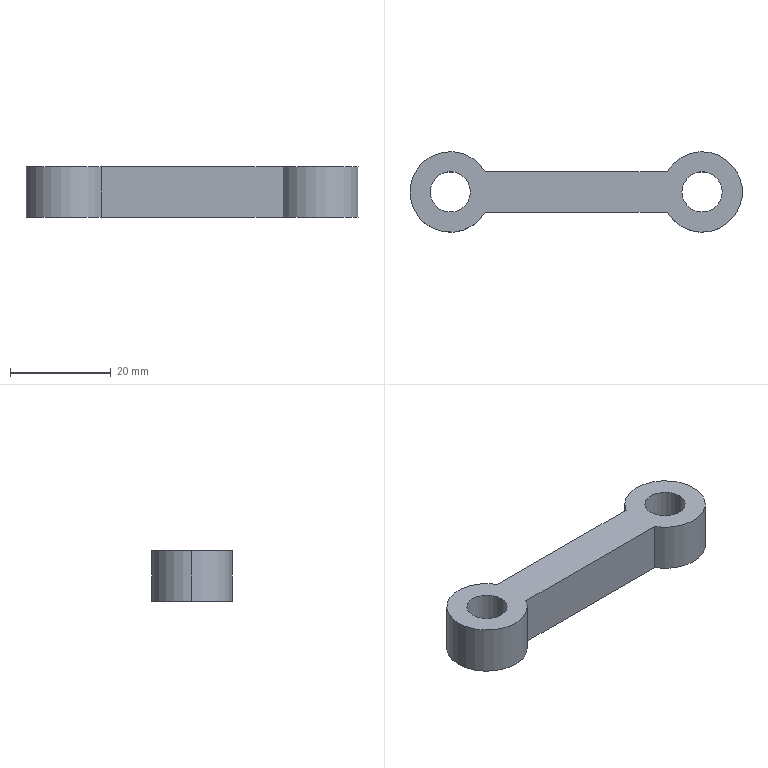Part | SolidWorks | features Extrusion 1 | 1 solid | 11 faces | box 66 x 16 x 10 mm | volume 5791 mm3 | cylinder 7 | plane 4 | commonest cylinder face diameters 8 x4 16 x3
STEP:
#1=CARTESIAN_POINT('',(46.,0.,10.));
#2=VERTEX_POINT('',#1);
#3=CARTESIAN_POINT('',(54.,0.,10.));
#4=VERTEX_POINT('',#3);
#5=CARTESIAN_POINT('',(50.,0.,10.));
#6=DIRECTION('',(0.,0.,1.));
#7=DIRECTION('',(1.,0.,0.));
#8=AXIS2_PLACEMENT_3D('',#5,#6,#7);
#9=CIRCLE('',#8,4.);
#10=EDGE_CURVE('',#2,#4,#9,.T.);
#11=ORIENTED_EDGE('',*,*,#10,.T.);
#12=CARTESIAN_POINT('',(54.,0.,0.));
#13=VERTEX_POINT('',#12);
#14=CARTESIAN_POINT('',(54.,0.,10.));
#15=DIRECTION('',(0.,0.,-1.));
#16=VECTOR('',#15,1000.);
#17=LINE('',#14,#16);
#18=EDGE_CURVE('',#4,#13,#17,.T.);
#19=ORIENTED_EDGE('',*,*,#18,.T.);
#20=CARTESIAN_POINT('',(46.,0.,0.));
#21=VERTEX_POINT('',#20);
#22=CARTESIAN_POINT('',(50.,0.,0.));
#23=DIRECTION('',(0.,0.,1.));
#24=DIRECTION('',(1.,0.,0.));
#25=AXIS2_PLACEMENT_3D('',#22,#23,#24);
#26=CIRCLE('',#25,4.);
#27=EDGE_CURVE('',#21,#13,#26,.T.);
#28=ORIENTED_EDGE('',*,*,#27,.F.);
#29=CARTESIAN_POINT('',(46.,0.,10.));
#30=DIRECTION('',(0.,0.,-1.));
#31=VECTOR('',#30,1000.);
#32=LINE('',#29,#31);
#33=EDGE_CURVE('',#2,#21,#32,.T.);
#34=ORIENTED_EDGE('',*,*,#33,.F.);
#35=EDGE_LOOP('',(#11,#19,#28,#34));
#36=FACE_OUTER_BOUND('',#35,.T.);
#37=CARTESIAN_POINT('',(50.,0.,10.));
#38=DIRECTION('',(0.,0.,-1.));
#39=DIRECTION('',(-1.,0.,0.));
#40=AXIS2_PLACEMENT_3D('',#37,#38,#39);
#41=CYLINDRICAL_SURFACE('',#40,4.);
#42=ADVANCED_FACE('',(#36),#41,.F.);
#43=CARTESIAN_POINT('',(-4.,0.,10.));
#44=VERTEX_POINT('',#43);
#45=CARTESIAN_POINT('',(4.,0.,10.));
#46=VERTEX_POINT('',#45);
#47=CARTESIAN_POINT('',(0.,0.,10.));
#48=DIRECTION('',(0.,0.,1.));
#49=DIRECTION('',(1.,0.,0.));
#50=AXIS2_PLACEMENT_3D('',#47,#48,#49);
#51=CIRCLE('',#50,4.);
#52=EDGE_CURVE('',#44,#46,#51,.T.);
#53=ORIENTED_EDGE('',*,*,#52,.T.);
#54=CARTESIAN_POINT('',(4.,0.,0.));
#55=VERTEX_POINT('',#54);
#56=CARTESIAN_POINT('',(4.,0.,10.));
#57=DIRECTION('',(0.,0.,-1.));
#58=VECTOR('',#57,1000.);
#59=LINE('',#56,#58);
#60=EDGE_CURVE('',#46,#55,#59,.T.);
#61=ORIENTED_EDGE('',*,*,#60,.T.);
#62=CARTESIAN_POINT('',(-4.,0.,0.));
#63=VERTEX_POINT('',#62);
#64=CARTESIAN_POINT('',(0.,0.,0.));
#65=DIRECTION('',(0.,0.,1.));
#66=DIRECTION('',(1.,0.,0.));
#67=AXIS2_PLACEMENT_3D('',#64,#65,#66);
#68=CIRCLE('',#67,4.);
#69=EDGE_CURVE('',#63,#55,#68,.T.);
#70=ORIENTED_EDGE('',*,*,#69,.F.);
#71=CARTESIAN_POINT('',(-4.,0.,10.));
#72=DIRECTION('',(0.,0.,-1.));
#73=VECTOR('',#72,1000.);
#74=LINE('',#71,#73);
#75=EDGE_CURVE('',#44,#63,#74,.T.);
#76=ORIENTED_EDGE('',*,*,#75,.F.);
#77=EDGE_LOOP('',(#53,#61,#70,#76));
#78=FACE_OUTER_BOUND('',#77,.T.);
#79=CARTESIAN_POINT('',(0.,0.,10.));
#80=DIRECTION('',(0.,0.,-1.));
#81=DIRECTION('',(-1.,0.,0.));
#82=AXIS2_PLACEMENT_3D('',#79,#80,#81);
#83=CYLINDRICAL_SURFACE('',#82,4.);
#84=ADVANCED_FACE('',(#78),#83,.F.);
#85=CARTESIAN_POINT('',(-8.,0.,10.));
#86=VERTEX_POINT('',#85);
#87=CARTESIAN_POINT('',(6.928,-4.,10.));
#88=VERTEX_POINT('',#87);
#89=CARTESIAN_POINT('',(0.,0.,10.));
#90=DIRECTION('',(0.,0.,1.));
#91=DIRECTION('',(1.,0.,0.));
#92=AXIS2_PLACEMENT_3D('',#89,#90,#91);
#93=CIRCLE('',#92,8.);
#94=EDGE_CURVE('',#86,#88,#93,.T.);
#95=ORIENTED_EDGE('',*,*,#94,.F.);
#96=CARTESIAN_POINT('',(-8.,0.,0.));
#97=VERTEX_POINT('',#96);
#98=CARTESIAN_POINT('',(-8.,0.,10.));
#99=DIRECTION('',(0.,0.,-1.));
#100=VECTOR('',#99,1000.);
#101=LINE('',#98,#100);
#102=EDGE_CURVE('',#86,#97,#101,.T.);
#103=ORIENTED_EDGE('',*,*,#102,.T.);
#104=CARTESIAN_POINT('',(6.928,-4.,0.));
#105=VERTEX_POINT('',#104);
#106=CARTESIAN_POINT('',(0.,0.,0.));
#107=DIRECTION('',(0.,0.,1.));
#108=DIRECTION('',(1.,0.,0.));
#109=AXIS2_PLACEMENT_3D('',#106,#107,#108);
#110=CIRCLE('',#109,8.);
#111=EDGE_CURVE('',#97,#105,#110,.T.);
#112=ORIENTED_EDGE('',*,*,#111,.T.);
#113=CARTESIAN_POINT('',(6.928,-4.,10.));
#114=DIRECTION('',(0.,0.,-1.));
#115=VECTOR('',#114,1000.);
#116=LINE('',#113,#115);
#117=EDGE_CURVE('',#88,#105,#116,.T.);
#118=ORIENTED_EDGE('',*,*,#117,.F.);
#119=EDGE_LOOP('',(#95,#103,#112,#118));
#120=FACE_OUTER_BOUND('',#119,.T.);
#121=CARTESIAN_POINT('',(0.,0.,10.));
#122=DIRECTION('',(0.,0.,-1.));
#123=DIRECTION('',(-1.,0.,0.));
#124=AXIS2_PLACEMENT_3D('',#121,#122,#123);
#125=CYLINDRICAL_SURFACE('',#124,8.);
#126=ADVANCED_FACE('',(#120),#125,.T.);
#127=ORIENTED_EDGE('',*,*,#52,.F.);
#128=CARTESIAN_POINT('',(0.,0.,10.));
#129=DIRECTION('',(0.,0.,1.));
#130=DIRECTION('',(1.,0.,0.));
#131=AXIS2_PLACEMENT_3D('',#128,#129,#130);
#132=CIRCLE('',#131,4.);
#133=EDGE_CURVE('',#46,#44,#132,.T.);
#134=ORIENTED_EDGE('',*,*,#133,.F.);
#135=EDGE_LOOP('',(#127,#134));
#136=FACE_BOUND('',#135,.T.);
#137=CARTESIAN_POINT('',(6.928,4.,10.));
#138=VERTEX_POINT('',#137);
#139=CARTESIAN_POINT('',(0.,0.,10.));
#140=DIRECTION('',(0.,0.,1.));
#141=DIRECTION('',(1.,0.,0.));
#142=AXIS2_PLACEMENT_3D('',#139,#140,#141);
#143=CIRCLE('',#142,8.);
#144=EDGE_CURVE('',#138,#86,#143,.T.);
#145=ORIENTED_EDGE('',*,*,#144,.T.);
#146=ORIENTED_EDGE('',*,*,#94,.T.);
#147=CARTESIAN_POINT('',(43.072,-4.,10.));
#148=VERTEX_POINT('',#147);
#149=CARTESIAN_POINT('',(6.928,-4.,10.));
#150=DIRECTION('',(1.,0.,0.));
#151=VECTOR('',#150,1000.);
#152=LINE('',#149,#151);
#153=EDGE_CURVE('',#88,#148,#152,.T.);
#154=ORIENTED_EDGE('',*,*,#153,.T.);
#155=CARTESIAN_POINT('',(43.072,4.,10.));
#156=VERTEX_POINT('',#155);
#157=CARTESIAN_POINT('',(50.,0.,10.));
#158=DIRECTION('',(0.,0.,1.));
#159=DIRECTION('',(1.,0.,0.));
#160=AXIS2_PLACEMENT_3D('',#157,#158,#159);
#161=CIRCLE('',#160,8.);
#162=EDGE_CURVE('',#148,#156,#161,.T.);
#163=ORIENTED_EDGE('',*,*,#162,.T.);
#164=CARTESIAN_POINT('',(6.928,4.,10.));
#165=DIRECTION('',(-1.,0.,0.));
#166=VECTOR('',#165,1000.);
#167=LINE('',#164,#166);
#168=EDGE_CURVE('',#156,#138,#167,.T.);
#169=ORIENTED_EDGE('',*,*,#168,.T.);
#170=EDGE_LOOP('',(#145,#146,#154,#163,#169));
#171=FACE_OUTER_BOUND('',#170,.T.);
#172=ORIENTED_EDGE('',*,*,#10,.F.);
#173=CARTESIAN_POINT('',(50.,0.,10.));
#174=DIRECTION('',(0.,0.,1.));
#175=DIRECTION('',(1.,0.,0.));
#176=AXIS2_PLACEMENT_3D('',#173,#174,#175);
#177=CIRCLE('',#176,4.);
#178=EDGE_CURVE('',#4,#2,#177,.T.);
#179=ORIENTED_EDGE('',*,*,#178,.F.);
#180=EDGE_LOOP('',(#172,#179));
#181=FACE_BOUND('',#180,.T.);
#182=CARTESIAN_POINT('',(0.,0.,10.));
#183=DIRECTION('',(0.,0.,1.));
#184=DIRECTION('',(1.,0.,0.));
#185=AXIS2_PLACEMENT_3D('',#182,#183,#184);
#186=PLANE('',#185);
#187=ADVANCED_FACE('',(#136,#171,#181),#186,.T.);
#188=CARTESIAN_POINT('',(6.928,4.,0.));
#189=VERTEX_POINT('',#188);
#190=CARTESIAN_POINT('',(0.,0.,0.));
#191=DIRECTION('',(0.,0.,1.));
#192=DIRECTION('',(1.,0.,0.));
#193=AXIS2_PLACEMENT_3D('',#190,#191,#192);
#194=CIRCLE('',#193,8.);
#195=EDGE_CURVE('',#189,#97,#194,.T.);
#196=ORIENTED_EDGE('',*,*,#195,.F.);
#197=CARTESIAN_POINT('',(43.072,4.,0.));
#198=VERTEX_POINT('',#197);
#199=CARTESIAN_POINT('',(6.928,4.,0.));
#200=DIRECTION('',(-1.,0.,0.));
#201=VECTOR('',#200,1000.);
#202=LINE('',#199,#201);
#203=EDGE_CURVE('',#198,#189,#202,.T.);
#204=ORIENTED_EDGE('',*,*,#203,.F.);
#205=CARTESIAN_POINT('',(43.072,-4.,0.));
#206=VERTEX_POINT('',#205);
#207=CARTESIAN_POINT('',(50.,0.,0.));
#208=DIRECTION('',(0.,0.,1.));
#209=DIRECTION('',(1.,0.,0.));
#210=AXIS2_PLACEMENT_3D('',#207,#208,#209);
#211=CIRCLE('',#210,8.);
#212=EDGE_CURVE('',#206,#198,#211,.T.);
#213=ORIENTED_EDGE('',*,*,#212,.F.);
#214=CARTESIAN_POINT('',(6.928,-4.,0.));
#215=DIRECTION('',(1.,0.,0.));
#216=VECTOR('',#215,1000.);
#217=LINE('',#214,#216);
#218=EDGE_CURVE('',#105,#206,#217,.T.);
#219=ORIENTED_EDGE('',*,*,#218,.F.);
#220=ORIENTED_EDGE('',*,*,#111,.F.);
#221=EDGE_LOOP('',(#196,#204,#213,#219,#220));
#222=FACE_OUTER_BOUND('',#221,.T.);
#223=ORIENTED_EDGE('',*,*,#69,.T.);
#224=CARTESIAN_POINT('',(0.,0.,0.));
#225=DIRECTION('',(0.,0.,1.));
#226=DIRECTION('',(1.,0.,0.));
#227=AXIS2_PLACEMENT_3D('',#224,#225,#226);
#228=CIRCLE('',#227,4.);
#229=EDGE_CURVE('',#55,#63,#228,.T.);
#230=ORIENTED_EDGE('',*,*,#229,.T.);
#231=EDGE_LOOP('',(#223,#230));
#232=FACE_BOUND('',#231,.T.);
#233=ORIENTED_EDGE('',*,*,#27,.T.);
#234=CARTESIAN_POINT('',(50.,0.,0.));
#235=DIRECTION('',(0.,0.,1.));
#236=DIRECTION('',(1.,0.,0.));
#237=AXIS2_PLACEMENT_3D('',#234,#235,#236);
#238=CIRCLE('',#237,4.);
#239=EDGE_CURVE('',#13,#21,#238,.T.);
#240=ORIENTED_EDGE('',*,*,#239,.T.);
#241=EDGE_LOOP('',(#233,#240));
#242=FACE_BOUND('',#241,.T.);
#243=CARTESIAN_POINT('',(0.,0.,0.));
#244=DIRECTION('',(0.,0.,1.));
#245=DIRECTION('',(1.,0.,0.));
#246=AXIS2_PLACEMENT_3D('',#243,#244,#245);
#247=PLANE('',#246);
#248=ADVANCED_FACE('',(#222,#232,#242),#247,.F.);
#249=ORIENTED_EDGE('',*,*,#102,.F.);
#250=ORIENTED_EDGE('',*,*,#144,.F.);
#251=CARTESIAN_POINT('',(6.928,4.,10.));
#252=DIRECTION('',(0.,0.,-1.));
#253=VECTOR('',#252,1000.);
#254=LINE('',#251,#253);
#255=EDGE_CURVE('',#138,#189,#254,.T.);
#256=ORIENTED_EDGE('',*,*,#255,.T.);
#257=ORIENTED_EDGE('',*,*,#195,.T.);
#258=EDGE_LOOP('',(#249,#250,#256,#257));
#259=FACE_OUTER_BOUND('',#258,.T.);
#260=CARTESIAN_POINT('',(0.,0.,10.));
#261=DIRECTION('',(0.,0.,-1.));
#262=DIRECTION('',(-1.,0.,0.));
#263=AXIS2_PLACEMENT_3D('',#260,#261,#262);
#264=CYLINDRICAL_SURFACE('',#263,8.);
#265=ADVANCED_FACE('',(#259),#264,.T.);
#266=ORIENTED_EDGE('',*,*,#218,.T.);
#267=CARTESIAN_POINT('',(43.072,-4.,10.));
#268=DIRECTION('',(0.,0.,-1.));
#269=VECTOR('',#268,1000.);
#270=LINE('',#267,#269);
#271=EDGE_CURVE('',#148,#206,#270,.T.);
#272=ORIENTED_EDGE('',*,*,#271,.F.);
#273=ORIENTED_EDGE('',*,*,#153,.F.);
#274=ORIENTED_EDGE('',*,*,#117,.T.);
#275=EDGE_LOOP('',(#266,#272,#273,#274));
#276=FACE_OUTER_BOUND('',#275,.T.);
#277=CARTESIAN_POINT('',(6.928,-4.,10.));
#278=DIRECTION('',(0.,1.,0.));
#279=DIRECTION('',(0.,0.,1.));
#280=AXIS2_PLACEMENT_3D('',#277,#278,#279);
#281=PLANE('',#280);
#282=ADVANCED_FACE('',(#276),#281,.F.);
#283=ORIENTED_EDGE('',*,*,#212,.T.);
#284=CARTESIAN_POINT('',(43.072,4.,10.));
#285=DIRECTION('',(0.,0.,-1.));
#286=VECTOR('',#285,1000.);
#287=LINE('',#284,#286);
#288=EDGE_CURVE('',#156,#198,#287,.T.);
#289=ORIENTED_EDGE('',*,*,#288,.F.);
#290=ORIENTED_EDGE('',*,*,#162,.F.);
#291=ORIENTED_EDGE('',*,*,#271,.T.);
#292=EDGE_LOOP('',(#283,#289,#290,#291));
#293=FACE_OUTER_BOUND('',#292,.T.);
#294=CARTESIAN_POINT('',(50.,0.,10.));
#295=DIRECTION('',(0.,0.,-1.));
#296=DIRECTION('',(-1.,0.,0.));
#297=AXIS2_PLACEMENT_3D('',#294,#295,#296);
#298=CYLINDRICAL_SURFACE('',#297,8.);
#299=ADVANCED_FACE('',(#293),#298,.T.);
#300=ORIENTED_EDGE('',*,*,#203,.T.);
#301=ORIENTED_EDGE('',*,*,#255,.F.);
#302=ORIENTED_EDGE('',*,*,#168,.F.);
#303=ORIENTED_EDGE('',*,*,#288,.T.);
#304=EDGE_LOOP('',(#300,#301,#302,#303));
#305=FACE_OUTER_BOUND('',#304,.T.);
#306=CARTESIAN_POINT('',(6.928,4.,10.));
#307=DIRECTION('',(0.,-1.,0.));
#308=DIRECTION('',(0.,0.,-1.));
#309=AXIS2_PLACEMENT_3D('',#306,#307,#308);
#310=PLANE('',#309);
#311=ADVANCED_FACE('',(#305),#310,.F.);
#312=ORIENTED_EDGE('',*,*,#60,.F.);
#313=ORIENTED_EDGE('',*,*,#133,.T.);
#314=ORIENTED_EDGE('',*,*,#75,.T.);
#315=ORIENTED_EDGE('',*,*,#229,.F.);
#316=EDGE_LOOP('',(#312,#313,#314,#315));
#317=FACE_OUTER_BOUND('',#316,.T.);
#318=CARTESIAN_POINT('',(0.,0.,10.));
#319=DIRECTION('',(0.,0.,-1.));
#320=DIRECTION('',(-1.,0.,0.));
#321=AXIS2_PLACEMENT_3D('',#318,#319,#320);
#322=CYLINDRICAL_SURFACE('',#321,4.);
#323=ADVANCED_FACE('',(#317),#322,.F.);
#324=ORIENTED_EDGE('',*,*,#18,.F.);
#325=ORIENTED_EDGE('',*,*,#178,.T.);
#326=ORIENTED_EDGE('',*,*,#33,.T.);
#327=ORIENTED_EDGE('',*,*,#239,.F.);
#328=EDGE_LOOP('',(#324,#325,#326,#327));
#329=FACE_OUTER_BOUND('',#328,.T.);
#330=CARTESIAN_POINT('',(50.,0.,10.));
#331=DIRECTION('',(0.,0.,-1.));
#332=DIRECTION('',(-1.,0.,0.));
#333=AXIS2_PLACEMENT_3D('',#330,#331,#332);
#334=CYLINDRICAL_SURFACE('',#333,4.);
#335=ADVANCED_FACE('',(#329),#334,.F.);
#336=CLOSED_SHELL('',(#42,#84,#126,#187,#248,#265,#282,#299,#311,#323,#335));
#337=MANIFOLD_SOLID_BREP('',#336);
#338=CARTESIAN_POINT('',(0.,0.,0.));
#339=DIRECTION('',(0.,0.,1.));
#340=DIRECTION('',(1.,0.,0.));
#341=AXIS2_PLACEMENT_3D('',#338,#339,#340);
#342=(LENGTH_UNIT()NAMED_UNIT(*)SI_UNIT(.MILLI.,.METRE.));
#343=UNCERTAINTY_MEASURE_WITH_UNIT(LENGTH_MEASURE(0.00001),#342,'','');
#344=(NAMED_UNIT(*)PLANE_ANGLE_UNIT()SI_UNIT($,.RADIAN.));
#345=(NAMED_UNIT(*)SI_UNIT($,.STERADIAN.)SOLID_ANGLE_UNIT());
#346=(GEOMETRIC_REPRESENTATION_CONTEXT(3)GLOBAL_UNCERTAINTY_ASSIGNED_CONTEXT((#343))GLOBAL_UNIT_ASSIGNED_CONTEXT((#342,#344,#345))REPRESENTATION_CONTEXT('',''));
#347=ADVANCED_BREP_SHAPE_REPRESENTATION('',(#337,#341),#346);